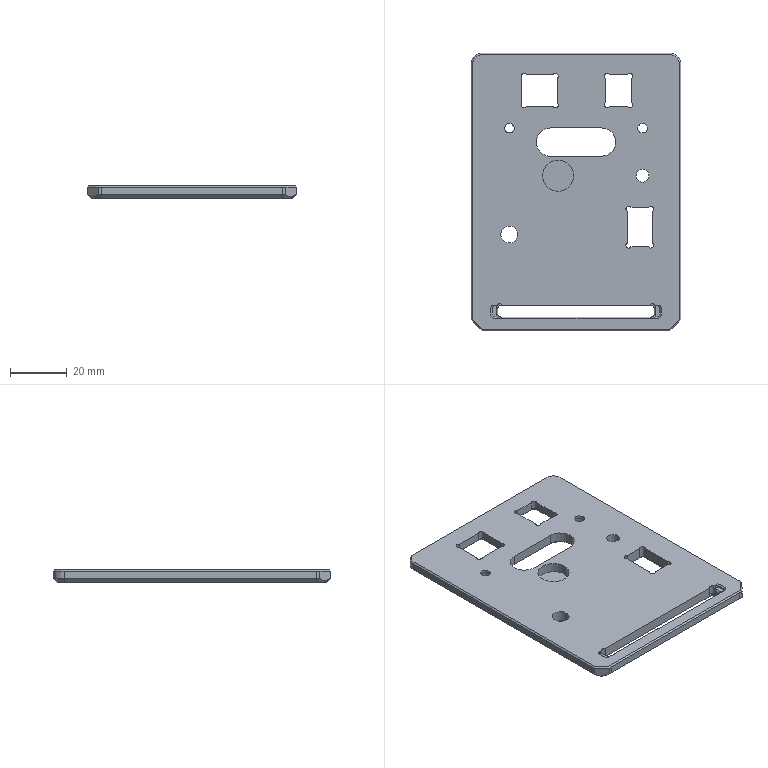Part | SolidWorks | features BaseBody 1 | 1 solid | 467 faces | box 74 x 98 x 4.5 mm | volume 27198 mm3 | plane 278 | spline 89 | cylinder 55 | cone 45 | commonest cylinder face diameters 2 x32 10 x7 3.4 x4 6.4 x4 4.5 x2 6 x2